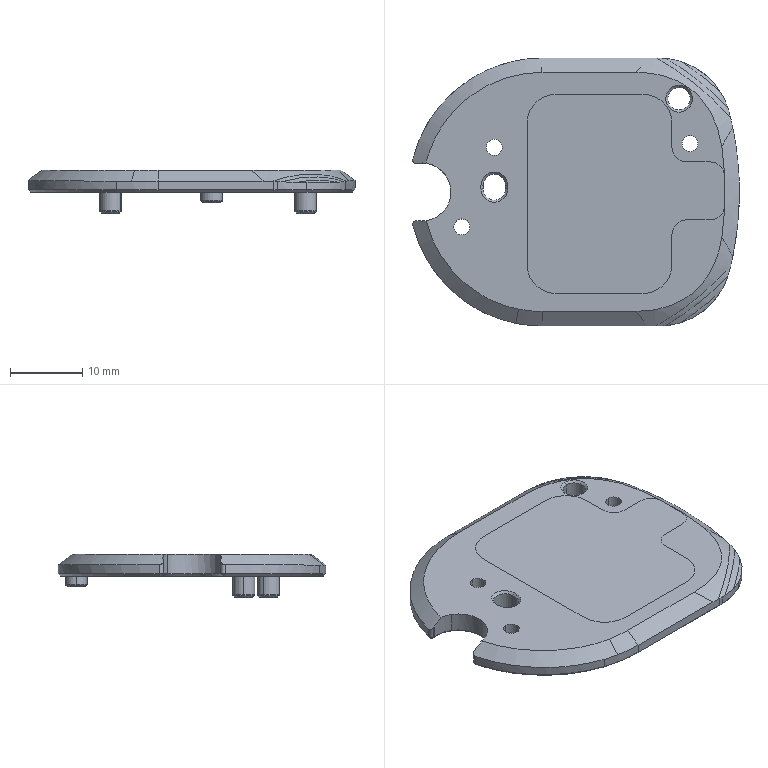Part | 2 solids | 316 faces | box 45.101 x 36.973 x 6 mm | volume 3995 mm3 | plane 139 | cylinder 77 | spline 36 | cone 35 | torus 27 | sphere 2 | commonest cylinder face diameters 0.4 x18 8 x11 1 x8 4 x8 2.2 x6 3 x6